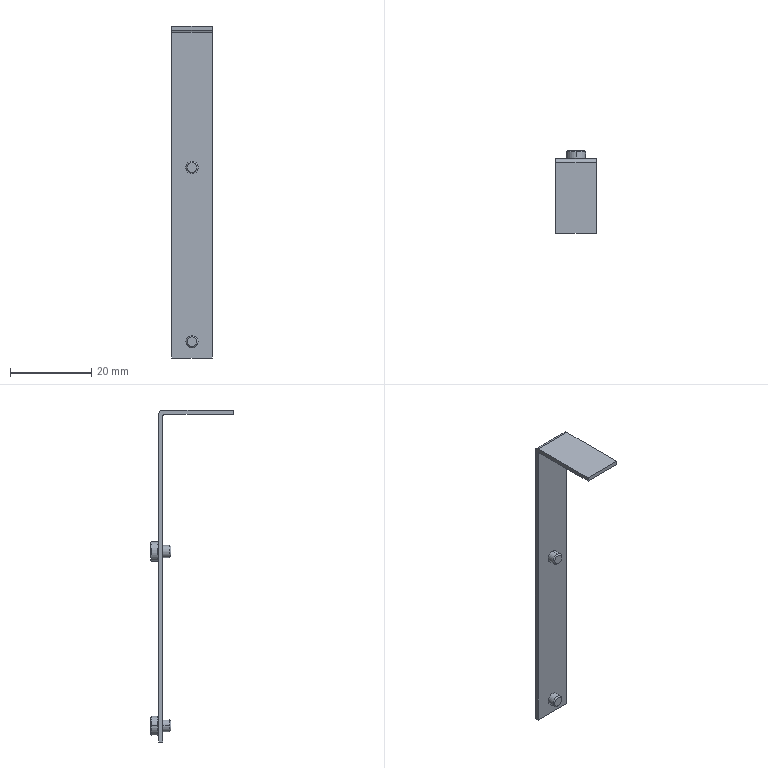Part | STEP file | Guide wheel mechanism revised.sldasm-Part-407 | 1 solid | 62 faces | box 10 x 20.4 x 81.9 mm | volume 1079 mm3 | plane 30 | cylinder 20 | cone 12 | commonest cylinder face diameters 3 x14 4.7 x4 1 x1 2 x1